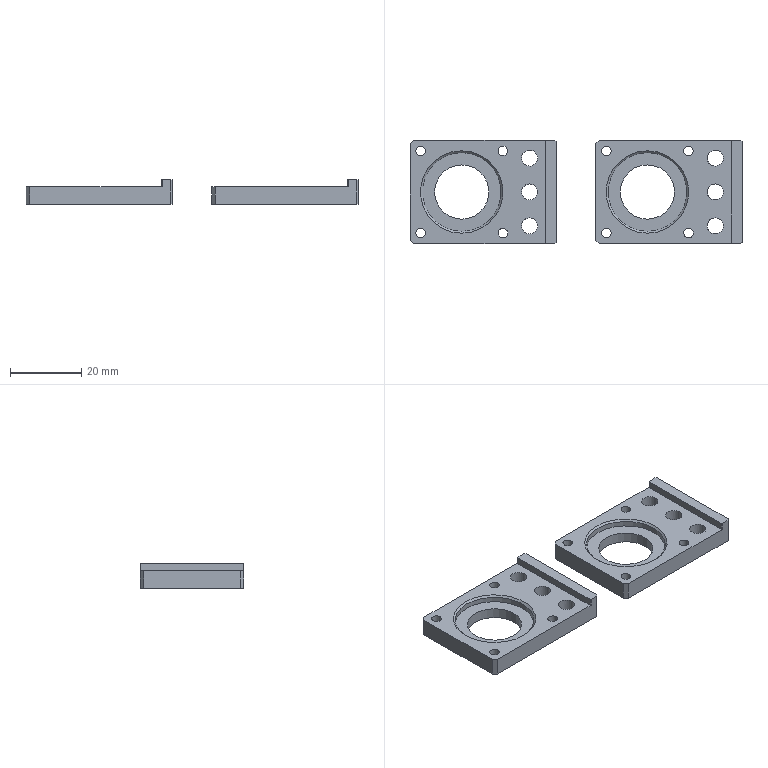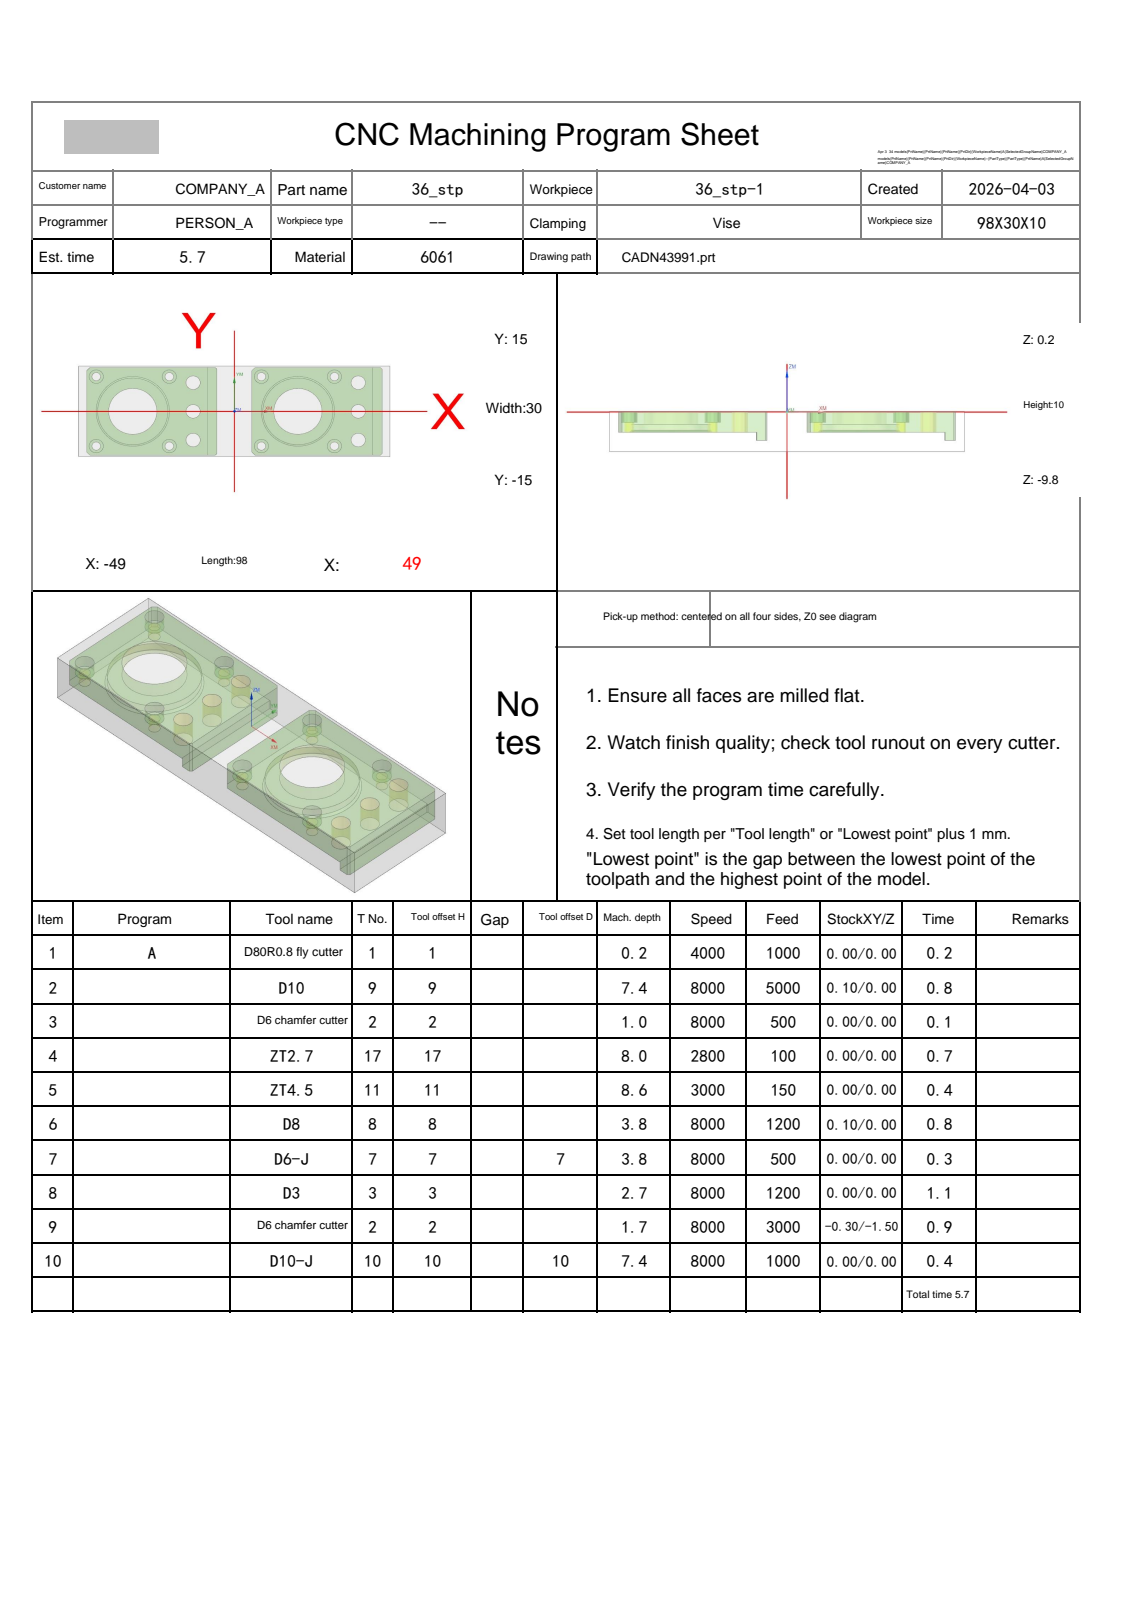NC program | NX | posted by the shop | part box 93 x 29 x 7 mm
Whole program, first 1395 of 1759 lines:
%
O0001
(Machine time: 7.58 MIN)
(===Total Tool:9===)
(T1=D80R0.8 fly cutter D=80.  R=0.8  D-  H01 Z=0.    )
(T9=D10     D=10.  R=0.   D-  H09 Z=-7.2  )
(T2=D6 chamfer cutter   D=6.   R=0.   D-  H02 Z=-1.5  )
(T17=ZT2.7  D=2.7  DR_a=120 D-  H17 Z=-7.78 )
(T11=ZT4.5  D=4.5  DR_a=118 D-  H11 Z=-8.35 )
(T8=D8      D=8.   R=0.   D-  H08 Z=-3.58 )
(T7=D6-J    D=6.   R=0.   D7  H07 Z=-3.58 )
(T3=D3      D=3.   R=0.   D3  H03 Z=-2.5  )
(T10=D10-J  D=10.  R=0.   D10 H10 Z=-7.2  )
G80 G90 G17 G49 G40
G91 G28 Z0
M01
N1 T01 M06
(D80R0.8 fly cutter  D=80. R=0.8 H=01 ce=0.00 di=0.00)
G00 G90 G54 X91.5 Y0.0 M03 S4000
G43 H01 Z20.
M08
Z2.
G01 Z0.0 F1000.
X86.5
X-86.5
X-91.5
Z2.
G00 Z20.
G91 G28 Z0.0
M05
M09
G91 G28 Z0.0
M01
N2 T09 M06
(D10  D=10. R=0. H=09 ce=0.10 di=0.00)
G00 G90 G54 X-25.75 Y-19.6 M03 S8000
G43 H09 Z20.
M08
Z.5
G01 X-45.5 Z.411 F5000.
G02 X-49.106 Y-18.106 Z.393 I0.0 J5.1
G01 X-50.106 Y-17.106 Z.386
G02 X-51.6 Y-13.5 Z.368 I3.606 J3.606
G01 Y13.5 Z.246
G02 X-50.106 Y17.106 Z.228 I5.1 J0.0
G01 X-49.106 Y18.106 Z.221
G02 X-45.5 Y19.6 Z.203 I3.606 J-3.606
G01 X-6. Z.025
G02 X-2.394 Y18.106 Z.007 I0.0 J-5.1
G01 X-1.894 Y17.606 Z.003
G02 X-.4 Y14. Z-.015 I-3.606 J-3.606
G01 Y-14. Z-.141
G02 X-1.894 Y-17.606 Z-.159 I-5.1 J0.0
G01 X-2.394 Y-18.106 Z-.163
G02 X-6. Y-19.6 Z-.181 I-3.606 J3.606
G01 X-45.5 Z-.359
G02 X-49.106 Y-18.106 Z-.377 I0.0 J5.1
G01 X-50.106 Y-17.106 Z-.384
G02 X-51.6 Y-13.5 Z-.402 I3.606 J3.606
G01 Y13.5 Z-.524
G02 X-50.106 Y17.106 Z-.542 I5.1 J0.0
G01 X-49.106 Y18.106 Z-.549
G02 X-45.5 Y19.6 Z-.567 I3.606 J-3.606
G01 X-6. Z-.745
G02 X-2.394 Y18.106 Z-.763 I0.0 J-5.1
G01 X-1.894 Y17.606 Z-.767
G02 X-.4 Y14. Z-.785 I-3.606 J-3.606
G01 Y-14. Z-.911
G02 X-1.894 Y-17.606 Z-.929 I-5.1 J0.0
G01 X-2.394 Y-18.106 Z-.933
G02 X-6. Y-19.6 Z-.951 I-3.606 J3.606
G01 X-45.5 Z-1.129
G02 X-49.106 Y-18.106 Z-1.147 I0.0 J5.1
G01 X-50.106 Y-17.106 Z-1.154
G02 X-51.6 Y-13.5 Z-1.172 I3.606 J3.606
G01 Y13.5 Z-1.294
G02 X-50.106 Y17.106 Z-1.312 I5.1 J0.0
G01 X-49.106 Y18.106 Z-1.319
G02 X-45.5 Y19.6 Z-1.337 I3.606 J-3.606
G01 X-6. Z-1.515
G02 X-2.394 Y18.106 Z-1.533 I0.0 J-5.1
G01 X-1.894 Y17.606 Z-1.537
G02 X-.4 Y14. Z-1.555 I-3.606 J-3.606
G01 Y-14. Z-1.681
G02 X-1.894 Y-17.606 Z-1.699 I-5.1 J0.0
G01 X-2.394 Y-18.106 Z-1.703
G02 X-6. Y-19.6 Z-1.721 I-3.606 J3.606
G01 X-45.5 Z-1.899
G02 X-49.106 Y-18.106 Z-1.917 I0.0 J5.1
G01 X-50.106 Y-17.106 Z-1.924
G02 X-51.6 Y-13.5 Z-1.942 I3.606 J3.606
G01 Y13.5 Z-2.064
G02 X-50.106 Y17.106 Z-2.082 I5.1 J0.0
G01 X-49.106 Y18.106 Z-2.089
G02 X-45.5 Y19.6 Z-2.107 I3.606 J-3.606
G01 X-6. Z-2.285
G02 X-2.394 Y18.106 Z-2.303 I0.0 J-5.1
G01 X-1.894 Y17.606 Z-2.307
G02 X-.4 Y14. Z-2.325 I-3.606 J-3.606
G01 Y-14. Z-2.451
G02 X-1.894 Y-17.606 Z-2.469 I-5.1 J0.0
G01 X-2.394 Y-18.106 Z-2.473
G02 X-6. Y-19.6 Z-2.491 I-3.606 J3.606
G01 X-45.5 Z-2.669
G02 X-49.106 Y-18.106 Z-2.687 I0.0 J5.1
G01 X-50.106 Y-17.106 Z-2.694
G02 X-51.6 Y-13.5 Z-2.712 I3.606 J3.606
G01 Y13.5 Z-2.834
G02 X-50.106 Y17.106 Z-2.852 I5.1 J0.0
G01 X-49.106 Y18.106 Z-2.859
G02 X-45.5 Y19.6 Z-2.877 I3.606 J-3.606
G01 X-6. Z-3.055
G02 X-2.394 Y18.106 Z-3.073 I0.0 J-5.1
G01 X-1.894 Y17.606 Z-3.077
G02 X-.4 Y14. Z-3.095 I-3.606 J-3.606
G01 Y-14. Z-3.221
G02 X-1.894 Y-17.606 Z-3.239 I-5.1 J0.0
G01 X-2.394 Y-18.106 Z-3.243
G02 X-6. Y-19.6 Z-3.261 I-3.606 J3.606
G01 X-45.5 Z-3.439
G02 X-49.106 Y-18.106 Z-3.457 I0.0 J5.1
G01 X-50.106 Y-17.106 Z-3.464
G02 X-51.6 Y-13.5 Z-3.482 I3.606 J3.606
G01 Y13.5 Z-3.604
G02 X-50.106 Y17.106 Z-3.622 I5.1 J0.0
G01 X-49.106 Y18.106 Z-3.629
G02 X-45.5 Y19.6 Z-3.647 I3.606 J-3.606
G01 X-6. Z-3.825
G02 X-2.394 Y18.106 Z-3.843 I0.0 J-5.1
G01 X-1.894 Y17.606 Z-3.847
G02 X-.4 Y14. Z-3.865 I-3.606 J-3.606
G01 Y-14. Z-3.991
G02 X-1.894 Y-17.606 Z-4.009 I-5.1 J0.0
G01 X-2.394 Y-18.106 Z-4.013
G02 X-6. Y-19.6 Z-4.031 I-3.606 J3.606
G01 X-45.5 Z-4.209
G02 X-49.106 Y-18.106 Z-4.227 I0.0 J5.1
G01 X-50.106 Y-17.106 Z-4.234
G02 X-51.6 Y-13.5 Z-4.252 I3.606 J3.606
G01 Y13.5 Z-4.374
G02 X-50.106 Y17.106 Z-4.392 I5.1 J0.0
G01 X-49.106 Y18.106 Z-4.399
G02 X-45.5 Y19.6 Z-4.417 I3.606 J-3.606
G01 X-6. Z-4.595
G02 X-2.394 Y18.106 Z-4.613 I0.0 J-5.1
G01 X-1.894 Y17.606 Z-4.617
G02 X-.4 Y14. Z-4.635 I-3.606 J-3.606
G01 Y-14. Z-4.761
G02 X-1.894 Y-17.606 Z-4.779 I-5.1 J0.0
G01 X-2.394 Y-18.106 Z-4.783
G02 X-6. Y-19.6 Z-4.801 I-3.606 J3.606
G01 X-45.5 Z-4.979
G02 X-49.106 Y-18.106 Z-4.997 I0.0 J5.1
G01 X-50.106 Y-17.106 Z-5.004
G02 X-51.6 Y-13.5 Z-5.022 I3.606 J3.606
G01 Y13.5 Z-5.144
G02 X-50.106 Y17.106 Z-5.162 I5.1 J0.0
G01 X-49.106 Y18.106 Z-5.169
G02 X-45.5 Y19.6 Z-5.187 I3.606 J-3.606
G01 X-6. Z-5.365
G02 X-2.394 Y18.106 Z-5.383 I0.0 J-5.1
G01 X-1.894 Y17.606 Z-5.387
G02 X-.4 Y14. Z-5.405 I-3.606 J-3.606
G01 Y-14. Z-5.531
G02 X-1.894 Y-17.606 Z-5.549 I-5.1 J0.0
G01 X-2.394 Y-18.106 Z-5.553
G02 X-6. Y-19.6 Z-5.571 I-3.606 J3.606
G01 X-45.5 Z-5.749
G02 X-49.106 Y-18.106 Z-5.767 I0.0 J5.1
G01 X-50.106 Y-17.106 Z-5.774
G02 X-51.6 Y-13.5 Z-5.792 I3.606 J3.606
G01 Y13.5 Z-5.914
G02 X-50.106 Y17.106 Z-5.932 I5.1 J0.0
G01 X-49.106 Y18.106 Z-5.939
G02 X-45.5 Y19.6 Z-5.957 I3.606 J-3.606
G01 X-6. Z-6.135
G02 X-2.394 Y18.106 Z-6.153 I0.0 J-5.1
G01 X-1.894 Y17.606 Z-6.157
G02 X-.4 Y14. Z-6.175 I-3.606 J-3.606
G01 Y-14. Z-6.301
G02 X-1.894 Y-17.606 Z-6.319 I-5.1 J0.0
G01 X-2.394 Y-18.106 Z-6.323
G02 X-6. Y-19.6 Z-6.341 I-3.606 J3.606
G01 X-45.5 Z-6.519
G02 X-49.106 Y-18.106 Z-6.537 I0.0 J5.1
G01 X-50.106 Y-17.106 Z-6.544
G02 X-51.6 Y-13.5 Z-6.562 I3.606 J3.606
G01 Y13.5 Z-6.684
G02 X-50.106 Y17.106 Z-6.702 I5.1 J0.0
G01 X-49.106 Y18.106 Z-6.709
G02 X-45.5 Y19.6 Z-6.727 I3.606 J-3.606
G01 X-6. Z-6.905
G02 X-2.394 Y18.106 Z-6.923 I0.0 J-5.1
G01 X-1.894 Y17.606 Z-6.927
G02 X-.4 Y14. Z-6.945 I-3.606 J-3.606
G01 Y-14. Z-7.071
G02 X-1.894 Y-17.606 Z-7.089 I-5.1 J0.0
G01 X-2.394 Y-18.106 Z-7.093
G02 X-6. Y-19.6 Z-7.111 I-3.606 J3.606
G01 X-25.75 Z-7.2
X-45.5
G02 X-49.106 Y-18.106 I0.0 J5.1
G01 X-50.106 Y-17.106
G02 X-51.6 Y-13.5 I3.606 J3.606
G01 Y13.5
G02 X-50.106 Y17.106 I5.1 J0.0
G01 X-49.106 Y18.106
G02 X-45.5 Y19.6 I3.606 J-3.606
G01 X-6.
G02 X-2.394 Y18.106 I0.0 J-5.1
G01 X-1.894 Y17.606
G02 X-.4 Y14. I-3.606 J-3.606
G01 Y-14.
G02 X-1.894 Y-17.606 I-5.1 J0.0
G01 X-2.394 Y-18.106
G02 X-6. Y-19.6 I-3.606 J3.606
G01 X-25.75
X-26.25
Z-6.2
G00 Z20.
X26.25
Z.5
G01 X6.5 Z.411
G02 X2.894 Y-18.106 Z.393 I0.0 J5.1
G01 X1.894 Y-17.106 Z.386
G02 X.4 Y-13.5 Z.368 I3.606 J3.606
G01 Y13.5 Z.246
G02 X1.894 Y17.106 Z.228 I5.1 J0.0
G01 X2.894 Y18.106 Z.221
G02 X6.5 Y19.6 Z.203 I3.606 J-3.606
G01 X46. Z.025
G02 X49.606 Y18.106 Z.007 I0.0 J-5.1
G01 X50.106 Y17.606 Z.003
G02 X51.6 Y14. Z-.015 I-3.606 J-3.606
G01 Y-14. Z-.141
G02 X50.106 Y-17.606 Z-.159 I-5.1 J0.0
G01 X49.606 Y-18.106 Z-.163
G02 X46. Y-19.6 Z-.181 I-3.606 J3.606
G01 X6.5 Z-.359
G02 X2.894 Y-18.106 Z-.377 I0.0 J5.1
G01 X1.894 Y-17.106 Z-.384
G02 X.4 Y-13.5 Z-.402 I3.606 J3.606
G01 Y13.5 Z-.524
G02 X1.894 Y17.106 Z-.542 I5.1 J0.0
G01 X2.894 Y18.106 Z-.549
G02 X6.5 Y19.6 Z-.567 I3.606 J-3.606
G01 X46. Z-.745
G02 X49.606 Y18.106 Z-.763 I0.0 J-5.1
G01 X50.106 Y17.606 Z-.767
G02 X51.6 Y14. Z-.785 I-3.606 J-3.606
G01 Y-14. Z-.911
G02 X50.106 Y-17.606 Z-.929 I-5.1 J0.0
G01 X49.606 Y-18.106 Z-.933
G02 X46. Y-19.6 Z-.951 I-3.606 J3.606
G01 X6.5 Z-1.129
G02 X2.894 Y-18.106 Z-1.147 I0.0 J5.1
G01 X1.894 Y-17.106 Z-1.154
G02 X.4 Y-13.5 Z-1.172 I3.606 J3.606
G01 Y13.5 Z-1.294
G02 X1.894 Y17.106 Z-1.312 I5.1 J0.0
G01 X2.894 Y18.106 Z-1.319
G02 X6.5 Y19.6 Z-1.337 I3.606 J-3.606
G01 X46. Z-1.515
G02 X49.606 Y18.106 Z-1.533 I0.0 J-5.1
G01 X50.106 Y17.606 Z-1.537
G02 X51.6 Y14. Z-1.555 I-3.606 J-3.606
G01 Y-14. Z-1.681
G02 X50.106 Y-17.606 Z-1.699 I-5.1 J0.0
G01 X49.606 Y-18.106 Z-1.703
G02 X46. Y-19.6 Z-1.721 I-3.606 J3.606
G01 X6.5 Z-1.899
G02 X2.894 Y-18.106 Z-1.917 I0.0 J5.1
G01 X1.894 Y-17.106 Z-1.924
G02 X.4 Y-13.5 Z-1.942 I3.606 J3.606
G01 Y13.5 Z-2.064
G02 X1.894 Y17.106 Z-2.082 I5.1 J0.0
G01 X2.894 Y18.106 Z-2.089
G02 X6.5 Y19.6 Z-2.107 I3.606 J-3.606
G01 X46. Z-2.285
G02 X49.606 Y18.106 Z-2.303 I0.0 J-5.1
G01 X50.106 Y17.606 Z-2.307
G02 X51.6 Y14. Z-2.325 I-3.606 J-3.606
G01 Y-14. Z-2.451
G02 X50.106 Y-17.606 Z-2.469 I-5.1 J0.0
G01 X49.606 Y-18.106 Z-2.473
G02 X46. Y-19.6 Z-2.491 I-3.606 J3.606
G01 X6.5 Z-2.669
G02 X2.894 Y-18.106 Z-2.687 I0.0 J5.1
G01 X1.894 Y-17.106 Z-2.694
G02 X.4 Y-13.5 Z-2.712 I3.606 J3.606
G01 Y13.5 Z-2.834
G02 X1.894 Y17.106 Z-2.852 I5.1 J0.0
G01 X2.894 Y18.106 Z-2.859
G02 X6.5 Y19.6 Z-2.877 I3.606 J-3.606
G01 X46. Z-3.055
G02 X49.606 Y18.106 Z-3.073 I0.0 J-5.1
G01 X50.106 Y17.606 Z-3.077
G02 X51.6 Y14. Z-3.095 I-3.606 J-3.606
G01 Y-14. Z-3.221
G02 X50.106 Y-17.606 Z-3.239 I-5.1 J0.0
G01 X49.606 Y-18.106 Z-3.243
G02 X46. Y-19.6 Z-3.261 I-3.606 J3.606
G01 X6.5 Z-3.439
G02 X2.894 Y-18.106 Z-3.457 I0.0 J5.1
G01 X1.894 Y-17.106 Z-3.464
G02 X.4 Y-13.5 Z-3.482 I3.606 J3.606
G01 Y13.5 Z-3.604
G02 X1.894 Y17.106 Z-3.622 I5.1 J0.0
G01 X2.894 Y18.106 Z-3.629
G02 X6.5 Y19.6 Z-3.647 I3.606 J-3.606
G01 X46. Z-3.825
G02 X49.606 Y18.106 Z-3.843 I0.0 J-5.1
G01 X50.106 Y17.606 Z-3.847
G02 X51.6 Y14. Z-3.865 I-3.606 J-3.606
G01 Y-14. Z-3.991
G02 X50.106 Y-17.606 Z-4.009 I-5.1 J0.0
G01 X49.606 Y-18.106 Z-4.013
G02 X46. Y-19.6 Z-4.031 I-3.606 J3.606
G01 X6.5 Z-4.209
G02 X2.894 Y-18.106 Z-4.227 I0.0 J5.1
G01 X1.894 Y-17.106 Z-4.234
G02 X.4 Y-13.5 Z-4.252 I3.606 J3.606
G01 Y13.5 Z-4.374
G02 X1.894 Y17.106 Z-4.392 I5.1 J0.0
G01 X2.894 Y18.106 Z-4.399
G02 X6.5 Y19.6 Z-4.417 I3.606 J-3.606
G01 X46. Z-4.595
G02 X49.606 Y18.106 Z-4.613 I0.0 J-5.1
G01 X50.106 Y17.606 Z-4.617
G02 X51.6 Y14. Z-4.635 I-3.606 J-3.606
G01 Y-14. Z-4.761
G02 X50.106 Y-17.606 Z-4.779 I-5.1 J0.0
G01 X49.606 Y-18.106 Z-4.783
G02 X46. Y-19.6 Z-4.801 I-3.606 J3.606
G01 X6.5 Z-4.979
G02 X2.894 Y-18.106 Z-4.997 I0.0 J5.1
G01 X1.894 Y-17.106 Z-5.004
G02 X.4 Y-13.5 Z-5.022 I3.606 J3.606
G01 Y13.5 Z-5.144
G02 X1.894 Y17.106 Z-5.162 I5.1 J0.0
G01 X2.894 Y18.106 Z-5.169
G02 X6.5 Y19.6 Z-5.187 I3.606 J-3.606
G01 X46. Z-5.365
G02 X49.606 Y18.106 Z-5.383 I0.0 J-5.1
G01 X50.106 Y17.606 Z-5.387
G02 X51.6 Y14. Z-5.405 I-3.606 J-3.606
G01 Y-14. Z-5.531
G02 X50.106 Y-17.606 Z-5.549 I-5.1 J0.0
G01 X49.606 Y-18.106 Z-5.553
G02 X46. Y-19.6 Z-5.571 I-3.606 J3.606
G01 X6.5 Z-5.749
G02 X2.894 Y-18.106 Z-5.767 I0.0 J5.1
G01 X1.894 Y-17.106 Z-5.774
G02 X.4 Y-13.5 Z-5.792 I3.606 J3.606
G01 Y13.5 Z-5.914
G02 X1.894 Y17.106 Z-5.932 I5.1 J0.0
G01 X2.894 Y18.106 Z-5.939
G02 X6.5 Y19.6 Z-5.957 I3.606 J-3.606
G01 X46. Z-6.135
G02 X49.606 Y18.106 Z-6.153 I0.0 J-5.1
G01 X50.106 Y17.606 Z-6.157
G02 X51.6 Y14. Z-6.175 I-3.606 J-3.606
G01 Y-14. Z-6.301
G02 X50.106 Y-17.606 Z-6.319 I-5.1 J0.0
G01 X49.606 Y-18.106 Z-6.323
G02 X46. Y-19.6 Z-6.341 I-3.606 J3.606
G01 X6.5 Z-6.519
G02 X2.894 Y-18.106 Z-6.537 I0.0 J5.1
G01 X1.894 Y-17.106 Z-6.544
G02 X.4 Y-13.5 Z-6.562 I3.606 J3.606
G01 Y13.5 Z-6.684
G02 X1.894 Y17.106 Z-6.702 I5.1 J0.0
G01 X2.894 Y18.106 Z-6.709
G02 X6.5 Y19.6 Z-6.727 I3.606 J-3.606
G01 X46. Z-6.905
G02 X49.606 Y18.106 Z-6.923 I0.0 J-5.1
G01 X50.106 Y17.606 Z-6.927
G02 X51.6 Y14. Z-6.945 I-3.606 J-3.606
G01 Y-14. Z-7.071
G02 X50.106 Y-17.606 Z-7.089 I-5.1 J0.0
G01 X49.606 Y-18.106 Z-7.093
G02 X46. Y-19.6 Z-7.111 I-3.606 J3.606
G01 X26.25 Z-7.2
X6.5
G02 X2.894 Y-18.106 I0.0 J5.1
G01 X1.894 Y-17.106
G02 X.4 Y-13.5 I3.606 J3.606
G01 Y13.5
G02 X1.894 Y17.106 I5.1 J0.0
G01 X2.894 Y18.106
G02 X6.5 Y19.6 I3.606 J-3.606
G01 X46.
G02 X49.606 Y18.106 I0.0 J-5.1
G01 X50.106 Y17.606
G02 X51.6 Y14. I-3.606 J-3.606
G01 Y-14.
G02 X50.106 Y-17.606 I-5.1 J0.0
G01 X49.606 Y-18.106
G02 X46. Y-19.6 I-3.606 J3.606
G01 X26.25
X25.75
Z-6.2
G00 Z20.
G91 G28 Z0.0
M05
M09
G91 G28 Z0.0
M01
N3 T02 M06
(D6 chamfer cutter  D=6. R=0. H=02 ce=0.00 di=0.00)
G00 G90 G54 X-43.5 Y-11.5 M03 S8000
G43 H02 Z20.
M08
G98 G81 X-43.5 Y-11.5 Z-.8 R1. F500.
Y11.5
X-32. Y0.0
X-20.5 Y11.5
X-13. Y9.5
Y0.0
X-20.5 Y-11.5
X-13. Y-9.5
X8.5 Y-11.5
X20. Y0.0
X31.5 Y-11.5
X39. Y-9.5
Y0.0
Y9.5
X31.5 Y11.5
X8.5
G80
G00 Z20.
G91 G28 Z0.0
M05
M09
G91 G28 Z0.0
M01
N4 T17 M06
(ZT2.7 D=2.7 DR_a=120 H=17)
G00 G90 G54 X-20.5 Y-11.5 M03 S2800
G43 H17 Z20.
M08
G98 G83 X-20.5 Y-11.5 Z-7.779 R1. F100. Q2.
X-43.5
Y11.5
X-20.5
X8.5
Y-11.5
X31.5
Y11.5
G80
G00 Z20.
G91 G28 Z0.0
M05
M09
G91 G28 Z0.0
M01
N5 T11 M06
(ZT4.5 D=4.5 DR_a=118 H=11)
G00 G90 G54 X-13. Y9.5 M03 S3000
G43 H11 Z20.
M08
G98 G83 X-13. Y9.5 Z-8.352 R1. F150. Q3.
Y0.0
Y-9.5
X39.
Y0.0
Y9.5
G80
G00 Z20.
G91 G28 Z0.0
M05
M09
G91 G28 Z0.0
M01
N6 T08 M06
(D8  D=8. R=0. H=08 ce=0.10 di=0.00)
G00 G90 G54 X-32. Y0.0 M03 S8000
G43 H08 Z20.
M08
Z.5
G03 X-30.25 Y-1.75 I1.75 J0.0 F1200.
X-28.5 Y0.0 I0.0 J1.75
X-28.5 Y0.0 Z.3 I-3.5 J0.0
X-28.5 Y0.0 Z.1 I-3.5 J0.0
X-28.5 Y0.0 Z-.1 I-3.5 J0.0
X-28.5 Y0.0 Z-.3 I-3.5 J0.0
X-28.5 Y0.0 Z-.5 I-3.5 J0.0
X-28.5 Y0.0 Z-.7 I-3.5 J0.0
X-28.5 Y0.0 Z-.9 I-3.5 J0.0
X-28.5 Y0.0 Z-1.1 I-3.5 J0.0
X-28.5 Y0.0 Z-1.3 I-3.5 J0.0
X-28.5 Y0.0 Z-1.5 I-3.5 J0.0
X-28.5 Y0.0 Z-1.7 I-3.5 J0.0
X-28.5 Y0.0 Z-1.9 I-3.5 J0.0
X-28.5 Y0.0 Z-2.1 I-3.5 J0.0
X-28.5 Y0.0 Z-2.3 I-3.5 J0.0
X-28.5 Y0.0 Z-2.5 I-3.5 J0.0
X-28.5 Y0.0 Z-2.7 I-3.5 J0.0
X-28.5 Y0.0 Z-2.9 I-3.5 J0.0
X-28.5 Y0.0 Z-3.1 I-3.5 J0.0
X-28.5 Y0.0 Z-3.3 I-3.5 J0.0
X-28.5 Y0.0 Z-3.5 I-3.5 J0.0
X-34.832 Y2.057 Z-3.58 I-3.5 J0.0
X-35.5 Y0.0 I2.832 J-2.057
X-32. Y-3.5 I3.5 J0.0
X-28.5 Y0.0 I0.0 J3.5
X-32. Y3.5 I-3.5 J0.0
X-34.832 Y2.057 I0.0 J-3.5
X-35.166 Y1.029 I1.416 J-1.029
X-33.416 Y-.721 I1.75 J0.0
X-32. Y0.0 I0.0 J1.75
G00 Z20.
X20.
Z.5
G03 X21.75 Y-1.75 I1.75 J0.0
X23.5 Y0.0 I0.0 J1.75
X23.5 Y0.0 Z.3 I-3.5 J0.0
X23.5 Y0.0 Z.1 I-3.5 J0.0
X23.5 Y0.0 Z-.1 I-3.5 J0.0
X23.5 Y0.0 Z-.3 I-3.5 J0.0
X23.5 Y0.0 Z-.5 I-3.5 J0.0
X23.5 Y0.0 Z-.7 I-3.5 J0.0
X23.5 Y0.0 Z-.9 I-3.5 J0.0
X23.5 Y0.0 Z-1.1 I-3.5 J0.0
X23.5 Y0.0 Z-1.3 I-3.5 J0.0
X23.5 Y0.0 Z-1.5 I-3.5 J0.0
X23.5 Y0.0 Z-1.7 I-3.5 J0.0
X23.5 Y0.0 Z-1.9 I-3.5 J0.0
X23.5 Y0.0 Z-2.1 I-3.5 J0.0
X23.5 Y0.0 Z-2.3 I-3.5 J0.0
X23.5 Y0.0 Z-2.5 I-3.5 J0.0
X23.5 Y0.0 Z-2.7 I-3.5 J0.0
X23.5 Y0.0 Z-2.9 I-3.5 J0.0
X23.5 Y0.0 Z-3.1 I-3.5 J0.0
X23.5 Y0.0 Z-3.3 I-3.5 J0.0
X23.5 Y0.0 Z-3.5 I-3.5 J0.0
X17.168 Y2.057 Z-3.58 I-3.5 J0.0
X16.5 Y0.0 I2.832 J-2.057
X20. Y-3.5 I3.5 J0.0
X23.5 Y0.0 I0.0 J3.5
X20. Y3.5 I-3.5 J0.0
X17.168 Y2.057 I0.0 J-3.5
X16.834 Y1.029 I1.416 J-1.029
X18.584 Y-.721 I1.75 J0.0
X20. Y0.0 I0.0 J1.75
G00 Z20.
G91 G28 Z0.0
M05
M09
G91 G28 Z0.0
M01
N7 T07 M06
(D6-J  D=6. R=0. H=07 ce=0.00 di=0.00)
G00 G90 G54 X-32. Y0.0 M03 S8000
G43 H07 Z20.
M08
Z.5
G41 D07
G01 X-31.116 Y-1.212 F500.
G03 X-29.455 Y-2.055 I1.66 J1.212
X-27.4 Y0.0 I0.0 J2.055
X-30.147 Y-4.21 Z-3.58 I-4.6 J0.0
X-27.4 Y0.0 I-1.853 J4.21
X-32. Y4.6 I-4.6 J0.0
X-36.6 Y0.0 I0.0 J-4.6
X-32. Y-4.6 I4.6 J0.0
X-30.147 Y-4.21 I0.0 J4.6
X-28.919 Y-2.329 I-.828 J1.881
X-30.535 Y-.321 I-2.055 J0.0
G01 G40 X-32. Y0.0
G00 Z20.
X20.
Z.5
G41 D07
G01 X20.884 Y-1.212
G03 X22.545 Y-2.055 I1.66 J1.212
X24.6 Y0.0 I0.0 J2.055
X21.853 Y-4.21 Z-3.58 I-4.6 J0.0
X24.6 Y0.0 I-1.853 J4.21
X20. Y4.6 I-4.6 J0.0
X15.4 Y0.0 I0.0 J-4.6
X20. Y-4.6 I4.6 J0.0
X21.853 Y-4.21 I0.0 J4.6
X23.081 Y-2.329 I-.828 J1.881
X21.465 Y-.321 I-2.055 J0.0
G01 G40 X20. Y0.0
G00 Z20.
G91 G28 Z0.0
M05
M09
G91 G28 Z0.0
M01
N8 T03 M06
(D3  D=3. R=0. H=03 ce=0.10 di=0.00)
G00 G90 G54 X-20.5 Y11.5 M03 S8000
G43 H03 Z20.
M08
Z.5
G03 X-20.175 Y11.175 I.325 J0.0 F1200.
X-19.85 Y11.5 I0.0 J.325
X-19.85 Y11.5 Z.4 I-.65 J0.0
X-19.85 Y11.5 Z.3 I-.65 J0.0
X-19.85 Y11.5 Z.2 I-.65 J0.0
X-19.85 Y11.5 Z.1 I-.65 J0.0
X-19.85 Y11.5 Z0.0 I-.65 J0.0
X-19.85 Y11.5 Z-.1 I-.65 J0.0
X-19.85 Y11.5 Z-.2 I-.65 J0.0
X-19.85 Y11.5 Z-.3 I-.65 J0.0
X-19.85 Y11.5 Z-.4 I-.65 J0.0
X-19.85 Y11.5 Z-.5 I-.65 J0.0
X-19.85 Y11.5 Z-.6 I-.65 J0.0
X-19.85 Y11.5 Z-.7 I-.65 J0.0
X-19.85 Y11.5 Z-.8 I-.65 J0.0
X-19.85 Y11.5 Z-.9 I-.65 J0.0
X-19.85 Y11.5 Z-1. I-.65 J0.0
X-19.85 Y11.5 Z-1.1 I-.65 J0.0
X-19.85 Y11.5 Z-1.2 I-.65 J0.0
X-19.85 Y11.5 Z-1.3 I-.65 J0.0
X-19.85 Y11.5 Z-1.4 I-.65 J0.0
X-19.85 Y11.5 Z-1.5 I-.65 J0.0
X-19.85 Y11.5 Z-1.6 I-.65 J0.0
X-19.85 Y11.5 Z-1.7 I-.65 J0.0
X-19.85 Y11.5 Z-1.8 I-.65 J0.0
X-19.85 Y11.5 Z-1.9 I-.65 J0.0
X-19.85 Y11.5 Z-2. I-.65 J0.0
X-19.85 Y11.5 Z-2.1 I-.65 J0.0
X-19.85 Y11.5 Z-2.2 I-.65 J0.0
X-19.85 Y11.5 Z-2.3 I-.65 J0.0
X-19.85 Y11.5 Z-2.4 I-.65 J0.0
X-19.85 Y11.5 Z-2.5 I-.65 J0.0
X-20.5 Y12.15 I-.65 J0.0
X-21.15 Y11.5 I0.0 J-.65
X-20.5 Y10.85 I.65 J0.0
X-19.85 Y11.5 I0.0 J.65
X-20.175 Y11.825 I-.325 J0.0
X-20.5 Y11.5 I0.0 J-.325
G00 Z20.
X-43.5
Z.5
G03 X-43.175 Y11.175 I.325 J0.0
X-42.85 Y11.5 I0.0 J.325
X-42.85 Y11.5 Z.4 I-.65 J0.0
X-42.85 Y11.5 Z.3 I-.65 J0.0
X-42.85 Y11.5 Z.2 I-.65 J0.0
X-42.85 Y11.5 Z.1 I-.65 J0.0
X-42.85 Y11.5 Z0.0 I-.65 J0.0
X-42.85 Y11.5 Z-.1 I-.65 J0.0
X-42.85 Y11.5 Z-.2 I-.65 J0.0
X-42.85 Y11.5 Z-.3 I-.65 J0.0
X-42.85 Y11.5 Z-.4 I-.65 J0.0
X-42.85 Y11.5 Z-.5 I-.65 J0.0
X-42.85 Y11.5 Z-.6 I-.65 J0.0
X-42.85 Y11.5 Z-.7 I-.65 J0.0
X-42.85 Y11.5 Z-.8 I-.65 J0.0
X-42.85 Y11.5 Z-.9 I-.65 J0.0
X-42.85 Y11.5 Z-1. I-.65 J0.0
X-42.85 Y11.5 Z-1.1 I-.65 J0.0
X-42.85 Y11.5 Z-1.2 I-.65 J0.0
X-42.85 Y11.5 Z-1.3 I-.65 J0.0
X-42.85 Y11.5 Z-1.4 I-.65 J0.0
X-42.85 Y11.5 Z-1.5 I-.65 J0.0
X-42.85 Y11.5 Z-1.6 I-.65 J0.0
X-42.85 Y11.5 Z-1.7 I-.65 J0.0
X-42.85 Y11.5 Z-1.8 I-.65 J0.0
X-42.85 Y11.5 Z-1.9 I-.65 J0.0
X-42.85 Y11.5 Z-2. I-.65 J0.0
X-42.85 Y11.5 Z-2.1 I-.65 J0.0
X-42.85 Y11.5 Z-2.2 I-.65 J0.0
X-42.85 Y11.5 Z-2.3 I-.65 J0.0
X-42.85 Y11.5 Z-2.4 I-.65 J0.0
X-42.85 Y11.5 Z-2.5 I-.65 J0.0
X-43.5 Y12.15 I-.65 J0.0
X-44.15 Y11.5 I0.0 J-.65
X-43.5 Y10.85 I.65 J0.0
X-42.85 Y11.5 I0.0 J.65
X-43.175 Y11.825 I-.325 J0.0
X-43.5 Y11.5 I0.0 J-.325
G00 Z20.
Y-11.5
Z.5
G03 X-43.175 Y-11.825 I.325 J0.0
X-42.85 Y-11.5 I0.0 J.325
X-42.85 Y-11.5 Z.4 I-.65 J0.0
X-42.85 Y-11.5 Z.3 I-.65 J0.0
X-42.85 Y-11.5 Z.2 I-.65 J0.0
X-42.85 Y-11.5 Z.1 I-.65 J0.0
X-42.85 Y-11.5 Z0.0 I-.65 J0.0
X-42.85 Y-11.5 Z-.1 I-.65 J0.0
X-42.85 Y-11.5 Z-.2 I-.65 J0.0
X-42.85 Y-11.5 Z-.3 I-.65 J0.0
X-42.85 Y-11.5 Z-.4 I-.65 J0.0
X-42.85 Y-11.5 Z-.5 I-.65 J0.0
X-42.85 Y-11.5 Z-.6 I-.65 J0.0
X-42.85 Y-11.5 Z-.7 I-.65 J0.0
X-42.85 Y-11.5 Z-.8 I-.65 J0.0
X-42.85 Y-11.5 Z-.9 I-.65 J0.0
X-42.85 Y-11.5 Z-1. I-.65 J0.0
X-42.85 Y-11.5 Z-1.1 I-.65 J0.0
X-42.85 Y-11.5 Z-1.2 I-.65 J0.0
X-42.85 Y-11.5 Z-1.3 I-.65 J0.0
X-42.85 Y-11.5 Z-1.4 I-.65 J0.0
X-42.85 Y-11.5 Z-1.5 I-.65 J0.0
X-42.85 Y-11.5 Z-1.6 I-.65 J0.0
X-42.85 Y-11.5 Z-1.7 I-.65 J0.0
X-42.85 Y-11.5 Z-1.8 I-.65 J0.0
X-42.85 Y-11.5 Z-1.9 I-.65 J0.0
X-42.85 Y-11.5 Z-2. I-.65 J0.0
X-42.85 Y-11.5 Z-2.1 I-.65 J0.0
X-42.85 Y-11.5 Z-2.2 I-.65 J0.0
X-42.85 Y-11.5 Z-2.3 I-.65 J0.0
X-42.85 Y-11.5 Z-2.4 I-.65 J0.0
X-42.85 Y-11.5 Z-2.5 I-.65 J0.0
X-43.5 Y-10.85 I-.65 J0.0
X-44.15 Y-11.5 I0.0 J-.65
X-43.5 Y-12.15 I.65 J0.0
X-42.85 Y-11.5 I0.0 J.65
X-43.175 Y-11.175 I-.325 J0.0
X-43.5 Y-11.5 I0.0 J-.325
G00 Z20.
X-20.5
Z.5
G03 X-20.175 Y-11.825 I.325 J0.0
X-19.85 Y-11.5 I0.0 J.325
X-19.85 Y-11.5 Z.4 I-.65 J0.0
X-19.85 Y-11.5 Z.3 I-.65 J0.0
X-19.85 Y-11.5 Z.2 I-.65 J0.0
X-19.85 Y-11.5 Z.1 I-.65 J0.0
X-19.85 Y-11.5 Z0.0 I-.65 J0.0
X-19.85 Y-11.5 Z-.1 I-.65 J0.0
X-19.85 Y-11.5 Z-.2 I-.65 J0.0
X-19.85 Y-11.5 Z-.3 I-.65 J0.0
X-19.85 Y-11.5 Z-.4 I-.65 J0.0
X-19.85 Y-11.5 Z-.5 I-.65 J0.0
X-19.85 Y-11.5 Z-.6 I-.65 J0.0
X-19.85 Y-11.5 Z-.7 I-.65 J0.0
X-19.85 Y-11.5 Z-.8 I-.65 J0.0
X-19.85 Y-11.5 Z-.9 I-.65 J0.0
X-19.85 Y-11.5 Z-1. I-.65 J0.0
X-19.85 Y-11.5 Z-1.1 I-.65 J0.0
X-19.85 Y-11.5 Z-1.2 I-.65 J0.0
X-19.85 Y-11.5 Z-1.3 I-.65 J0.0
X-19.85 Y-11.5 Z-1.4 I-.65 J0.0
X-19.85 Y-11.5 Z-1.5 I-.65 J0.0
X-19.85 Y-11.5 Z-1.6 I-.65 J0.0
X-19.85 Y-11.5 Z-1.7 I-.65 J0.0
X-19.85 Y-11.5 Z-1.8 I-.65 J0.0
X-19.85 Y-11.5 Z-1.9 I-.65 J0.0
X-19.85 Y-11.5 Z-2. I-.65 J0.0
X-19.85 Y-11.5 Z-2.1 I-.65 J0.0
X-19.85 Y-11.5 Z-2.2 I-.65 J0.0
X-19.85 Y-11.5 Z-2.3 I-.65 J0.0
X-19.85 Y-11.5 Z-2.4 I-.65 J0.0
X-19.85 Y-11.5 Z-2.5 I-.65 J0.0
X-20.5 Y-10.85 I-.65 J0.0
X-21.15 Y-11.5 I0.0 J-.65
X-20.5 Y-12.15 I.65 J0.0
X-19.85 Y-11.5 I0.0 J.65
X-20.175 Y-11.175 I-.325 J0.0
X-20.5 Y-11.5 I0.0 J-.325
G00 Z20.
X8.5
Z.5
G03 X8.825 Y-11.825 I.325 J0.0
X9.15 Y-11.5 I0.0 J.325
X9.15 Y-11.5 Z.4 I-.65 J0.0
X9.15 Y-11.5 Z.3 I-.65 J0.0
X9.15 Y-11.5 Z.2 I-.65 J0.0
X9.15 Y-11.5 Z.1 I-.65 J0.0
X9.15 Y-11.5 Z0.0 I-.65 J0.0
X9.15 Y-11.5 Z-.1 I-.65 J0.0
X9.15 Y-11.5 Z-.2 I-.65 J0.0
X9.15 Y-11.5 Z-.3 I-.65 J0.0
X9.15 Y-11.5 Z-.4 I-.65 J0.0
X9.15 Y-11.5 Z-.5 I-.65 J0.0
X9.15 Y-11.5 Z-.6 I-.65 J0.0
X9.15 Y-11.5 Z-.7 I-.65 J0.0
X9.15 Y-11.5 Z-.8 I-.65 J0.0
X9.15 Y-11.5 Z-.9 I-.65 J0.0
X9.15 Y-11.5 Z-1. I-.65 J0.0
X9.15 Y-11.5 Z-1.1 I-.65 J0.0
X9.15 Y-11.5 Z-1.2 I-.65 J0.0
X9.15 Y-11.5 Z-1.3 I-.65 J0.0
X9.15 Y-11.5 Z-1.4 I-.65 J0.0
X9.15 Y-11.5 Z-1.5 I-.65 J0.0
X9.15 Y-11.5 Z-1.6 I-.65 J0.0
X9.15 Y-11.5 Z-1.7 I-.65 J0.0
X9.15 Y-11.5 Z-1.8 I-.65 J0.0
X9.15 Y-11.5 Z-1.9 I-.65 J0.0
X9.15 Y-11.5 Z-2. I-.65 J0.0
X9.15 Y-11.5 Z-2.1 I-.65 J0.0
X9.15 Y-11.5 Z-2.2 I-.65 J0.0
X9.15 Y-11.5 Z-2.3 I-.65 J0.0
X9.15 Y-11.5 Z-2.4 I-.65 J0.0
X9.15 Y-11.5 Z-2.5 I-.65 J0.0
X8.5 Y-10.85 I-.65 J0.0
X7.85 Y-11.5 I0.0 J-.65
X8.5 Y-12.15 I.65 J0.0
X9.15 Y-11.5 I0.0 J.65
X8.825 Y-11.175 I-.325 J0.0
X8.5 Y-11.5 I0.0 J-.325
G00 Z20.
Y11.5
Z.5
G03 X8.825 Y11.175 I.325 J0.0
X9.15 Y11.5 I0.0 J.325
X9.15 Y11.5 Z.4 I-.65 J0.0
X9.15 Y11.5 Z.3 I-.65 J0.0
X9.15 Y11.5 Z.2 I-.65 J0.0
X9.15 Y11.5 Z.1 I-.65 J0.0
X9.15 Y11.5 Z0.0 I-.65 J0.0
X9.15 Y11.5 Z-.1 I-.65 J0.0
X9.15 Y11.5 Z-.2 I-.65 J0.0
X9.15 Y11.5 Z-.3 I-.65 J0.0
X9.15 Y11.5 Z-.4 I-.65 J0.0
X9.15 Y11.5 Z-.5 I-.65 J0.0
X9.15 Y11.5 Z-.6 I-.65 J0.0
X9.15 Y11.5 Z-.7 I-.65 J0.0
X9.15 Y11.5 Z-.8 I-.65 J0.0
X9.15 Y11.5 Z-.9 I-.65 J0.0
X9.15 Y11.5 Z-1. I-.65 J0.0
X9.15 Y11.5 Z-1.1 I-.65 J0.0
X9.15 Y11.5 Z-1.2 I-.65 J0.0
X9.15 Y11.5 Z-1.3 I-.65 J0.0
X9.15 Y11.5 Z-1.4 I-.65 J0.0
X9.15 Y11.5 Z-1.5 I-.65 J0.0
X9.15 Y11.5 Z-1.6 I-.65 J0.0
X9.15 Y11.5 Z-1.7 I-.65 J0.0
X9.15 Y11.5 Z-1.8 I-.65 J0.0
X9.15 Y11.5 Z-1.9 I-.65 J0.0
X9.15 Y11.5 Z-2. I-.65 J0.0
X9.15 Y11.5 Z-2.1 I-.65 J0.0
X9.15 Y11.5 Z-2.2 I-.65 J0.0
X9.15 Y11.5 Z-2.3 I-.65 J0.0
X9.15 Y11.5 Z-2.4 I-.65 J0.0
X9.15 Y11.5 Z-2.5 I-.65 J0.0
X8.5 Y12.15 I-.65 J0.0
X7.85 Y11.5 I0.0 J-.65
X8.5 Y10.85 I.65 J0.0
X9.15 Y11.5 I0.0 J.65
X8.825 Y11.825 I-.325 J0.0
X8.5 Y11.5 I0.0 J-.325
G00 Z20.
X31.5
Z.5
G03 X31.825 Y11.175 I.325 J0.0
X32.15 Y11.5 I0.0 J.325
X32.15 Y11.5 Z.4 I-.65 J0.0
X32.15 Y11.5 Z.3 I-.65 J0.0
X32.15 Y11.5 Z.2 I-.65 J0.0
X32.15 Y11.5 Z.1 I-.65 J0.0
X32.15 Y11.5 Z0.0 I-.65 J0.0
X32.15 Y11.5 Z-.1 I-.65 J0.0
X32.15 Y11.5 Z-.2 I-.65 J0.0
X32.15 Y11.5 Z-.3 I-.65 J0.0
X32.15 Y11.5 Z-.4 I-.65 J0.0
X32.15 Y11.5 Z-.5 I-.65 J0.0
X32.15 Y11.5 Z-.6 I-.65 J0.0
X32.15 Y11.5 Z-.7 I-.65 J0.0
X32.15 Y11.5 Z-.8 I-.65 J0.0
X32.15 Y11.5 Z-.9 I-.65 J0.0
X32.15 Y11.5 Z-1. I-.65 J0.0
X32.15 Y11.5 Z-1.1 I-.65 J0.0
X32.15 Y11.5 Z-1.2 I-.65 J0.0
X32.15 Y11.5 Z-1.3 I-.65 J0.0
X32.15 Y11.5 Z-1.4 I-.65 J0.0
X32.15 Y11.5 Z-1.5 I-.65 J0.0
X32.15 Y11.5 Z-1.6 I-.65 J0.0
X32.15 Y11.5 Z-1.7 I-.65 J0.0
X32.15 Y11.5 Z-1.8 I-.65 J0.0
X32.15 Y11.5 Z-1.9 I-.65 J0.0
X32.15 Y11.5 Z-2. I-.65 J0.0
X32.15 Y11.5 Z-2.1 I-.65 J0.0
X32.15 Y11.5 Z-2.2 I-.65 J0.0
X32.15 Y11.5 Z-2.3 I-.65 J0.0
X32.15 Y11.5 Z-2.4 I-.65 J0.0
X32.15 Y11.5 Z-2.5 I-.65 J0.0
X31.5 Y12.15 I-.65 J0.0
X30.85 Y11.5 I0.0 J-.65
X31.5 Y10.85 I.65 J0.0
X32.15 Y11.5 I0.0 J.65
X31.825 Y11.825 I-.325 J0.0
X31.5 Y11.5 I0.0 J-.325
G00 Z20.
Y-11.5
Z.5
G03 X31.825 Y-11.825 I.325 J0.0
X32.15 Y-11.5 I0.0 J.325
X32.15 Y-11.5 Z.4 I-.65 J0.0
X32.15 Y-11.5 Z.3 I-.65 J0.0
X32.15 Y-11.5 Z.2 I-.65 J0.0
X32.15 Y-11.5 Z.1 I-.65 J0.0
X32.15 Y-11.5 Z0.0 I-.65 J0.0
X32.15 Y-11.5 Z-.1 I-.65 J0.0
X32.15 Y-11.5 Z-.2 I-.65 J0.0
X32.15 Y-11.5 Z-.3 I-.65 J0.0
X32.15 Y-11.5 Z-.4 I-.65 J0.0
X32.15 Y-11.5 Z-.5 I-.65 J0.0
X32.15 Y-11.5 Z-.6 I-.65 J0.0
X32.15 Y-11.5 Z-.7 I-.65 J0.0
X32.15 Y-11.5 Z-.8 I-.65 J0.0
X32.15 Y-11.5 Z-.9 I-.65 J0.0
X32.15 Y-11.5 Z-1. I-.65 J0.0
X32.15 Y-11.5 Z-1.1 I-.65 J0.0
X32.15 Y-11.5 Z-1.2 I-.65 J0.0
X32.15 Y-11.5 Z-1.3 I-.65 J0.0
X32.15 Y-11.5 Z-1.4 I-.65 J0.0
X32.15 Y-11.5 Z-1.5 I-.65 J0.0
X32.15 Y-11.5 Z-1.6 I-.65 J0.0
X32.15 Y-11.5 Z-1.7 I-.65 J0.0
X32.15 Y-11.5 Z-1.8 I-.65 J0.0
X32.15 Y-11.5 Z-1.9 I-.65 J0.0
X32.15 Y-11.5 Z-2. I-.65 J0.0
X32.15 Y-11.5 Z-2.1 I-.65 J0.0
X32.15 Y-11.5 Z-2.2 I-.65 J0.0
X32.15 Y-11.5 Z-2.3 I-.65 J0.0
X32.15 Y-11.5 Z-2.4 I-.65 J0.0
X32.15 Y-11.5 Z-2.5 I-.65 J0.0
X31.5 Y-10.85 I-.65 J0.0
X30.85 Y-11.5 I0.0 J-.65
X31.5 Y-12.15 I.65 J0.0
X32.15 Y-11.5 I0.0 J.65
X31.825 Y-11.175 I-.325 J0.0
X31.5 Y-11.5 I0.0 J-.325
G00 Z20.
G00 G90 X-20.5 Y11.5 M03 S8000
Z20.
Z.5
G41 D03
G01 X-20.4 Y11.327 F500.
G03 X-20.098 Y11.152 I.302 J.173
X-19.75 Y11.5 I0.0 J.348
X-21.107 Y11.059 Z-2.5 I-.75 J0.0
X-20.5 Y10.75 I.607 J.441
X-19.75 Y11.5 I0.0 J.75
X-20.5 Y12.25 I-.75 J0.0
X-21.25 Y11.5 I0.0 J-.75
X-21.107 Y11.059 I.75 J0.0
X-20.825 Y10.916 I.282 J.205
X-20.477 Y11.264 I0.0 J.348
G01 X-20.479 Y11.301
G40 X-20.5 Y11.5
G00 Z20.
X-43.5
Z.5
G41 D03
G01 X-43.4 Y11.327
G03 X-43.098 Y11.152 I.302 J.173
X-42.75 Y11.5 I0.0 J.348
X-44.107 Y11.059 Z-2.5 I-.75 J0.0
X-43.5 Y10.75 I.607 J.441
X-42.75 Y11.5 I0.0 J.75
X-43.5 Y12.25 I-.75 J0.0
X-44.25 Y11.5 I0.0 J-.75
X-44.107 Y11.059 I.75 J0.0
X-43.825 Y10.916 I.282 J.205
X-43.477 Y11.264 I0.0 J.348
G01 X-43.479 Y11.301
G40 X-43.5 Y11.5
G00 Z20.
Y-11.5
Z.5
G41 D03
G01 X-43.4 Y-11.673
G03 X-43.098 Y-11.848 I.302 J.173
X-42.75 Y-11.5 I0.0 J.348
X-44.107 Y-11.941 Z-2.5 I-.75 J0.0
X-43.5 Y-12.25 I.607 J.441
X-42.75 Y-11.5 I0.0 J.75
X-43.5 Y-10.75 I-.75 J0.0
X-44.25 Y-11.5 I0.0 J-.75
X-44.107 Y-11.941 I.75 J0.0
X-43.825 Y-12.084 I.282 J.205
X-43.477 Y-11.736 I0.0 J.348
G01 X-43.479 Y-11.699
G40 X-43.5 Y-11.5
G00 Z20.
X-20.5
Z.5
G41 D03
G01 X-20.4 Y-11.673
G03 X-20.098 Y-11.848 I.302 J.173
X-19.75 Y-11.5 I0.0 J.348
X-21.107 Y-11.941 Z-2.5 I-.75 J0.0
X-20.5 Y-12.25 I.607 J.441
X-19.75 Y-11.5 I0.0 J.75
X-20.5 Y-10.75 I-.75 J0.0
X-21.25 Y-11.5 I0.0 J-.75
X-21.107 Y-11.941 I.75 J0.0
X-20.825 Y-12.084 I.282 J.205
X-20.477 Y-11.736 I0.0 J.348
G01 X-20.479 Y-11.699
G40 X-20.5 Y-11.5
G00 Z20.
X8.5
Z.5
G41 D03
G01 X8.6 Y-11.673
G03 X8.902 Y-11.848 I.302 J.173
X9.25 Y-11.5 I0.0 J.348
X7.893 Y-11.941 Z-2.5 I-.75 J0.0
X8.5 Y-12.25 I.607 J.441
X9.25 Y-11.5 I0.0 J.75
X8.5 Y-10.75 I-.75 J0.0
X7.75 Y-11.5 I0.0 J-.75
X7.893 Y-11.941 I.75 J0.0
X8.175 Y-12.084 I.282 J.205
X8.523 Y-11.736 I0.0 J.348
G01 X8.521 Y-11.699
G40 X8.5 Y-11.5
G00 Z20.
Y11.5
Z.5
G41 D03
G01 X8.6 Y11.327
G03 X8.902 Y11.152 I.302 J.173
X9.25 Y11.5 I0.0 J.348
X7.893 Y11.059 Z-2.5 I-.75 J0.0
X8.5 Y10.75 I.607 J.441
X9.25 Y11.5 I0.0 J.75
X8.5 Y12.25 I-.75 J0.0
X7.75 Y11.5 I0.0 J-.75
X7.893 Y11.059 I.75 J0.0
X8.175 Y10.916 I.282 J.205
X8.523 Y11.264 I0.0 J.348
G01 X8.521 Y11.301
G40 X8.5 Y11.5
G00 Z20.
X31.5
Z.5
G41 D03
G01 X31.6 Y11.327
G03 X31.902 Y11.152 I.302 J.173
X32.25 Y11.5 I0.0 J.348
X30.893 Y11.059 Z-2.5 I-.75 J0.0
X31.5 Y10.75 I.607 J.441
X32.25 Y11.5 I0.0 J.75
X31.5 Y12.25 I-.75 J0.0
X30.75 Y11.5 I0.0 J-.75
X30.893 Y11.059 I.75 J0.0
X31.175 Y10.916 I.282 J.205
X31.523 Y11.264 I0.0 J.348
G01 X31.521 Y11.301
G40 X31.5 Y11.5
G00 Z20.
Y-11.5
Z.5
G41 D03
G01 X31.6 Y-11.673
G03 X31.902 Y-11.848 I.302 J.173
X32.25 Y-11.5 I0.0 J.348
X30.893 Y-11.941 Z-2.5 I-.75 J0.0
X31.5 Y-12.25 I.607 J.441
X32.25 Y-11.5 I0.0 J.75
X31.5 Y-10.75 I-.75 J0.0
X30.75 Y-11.5 I0.0 J-.75
X30.893 Y-11.941 I.75 J0.0
X31.175 Y-12.084 I.282 J.205
X31.523 Y-11.736 I0.0 J.348
G01 X31.521 Y-11.699
G40 X31.5 Y-11.5
G00 Z20.
G91 G28 Z0.0
M05
M09
G91 G28 Z0.0
M01
N9 T02 M06
(D6 chamfer cutter  D=6. R=0. H=02 ce=0.00 di=0.00)
G00 G90 G54 X26. Y16.628 M03 S8000
G43 H02 Z20.
M08
Z2.099
G01 Z-1.499 F3000.
G03 X25.92 Y16.328 I.52 J-.3
X26.22 Y15.808 I.6 J0.0
G01 X26.25 Y15.8
X46.
X46.254 Y15.775
X46.497 Y15.701
X46.722 Y15.581
X46.919 Y15.419
X47.419 Y14.919
X47.581 Y14.722
X47.701 Y14.497
X47.775 Y14.254
X47.8 Y14.
Y-14.
X47.775 Y-14.254
X47.701 Y-14.497
X47.581 Y-14.722
X47.419 Y-14.919
X46.919 Y-15.419
X46.722 Y-15.581
X46.497 Y-15.701
X46.254 Y-15.775
X46. Y-15.8
X6.5
X6.246 Y-15.775
X6.003 Y-15.701
X5.778 Y-15.581
X5.581 Y-15.419
X4.581 Y-14.419
X4.419 Y-14.222
X4.299 Y-13.997
X4.225 Y-13.754
X4.2 Y-13.5
Y13.5
X4.225 Y13.754
X4.299 Y13.997
X4.419 Y14.222
X4.581 Y14.419
X5.581 Y15.419
X5.778 Y15.581
X6.003 Y15.701
X6.246 Y15.775
X6.5 Y15.8
X26.25
X26.28 Y15.808
G03 X26.58 Y16.328 I-.3 J.52
X26.5 Y16.628 I-.6 J0.0
G01 Z2.099
G00 Z20.
X14.513 Y.293
Z2.13
G01 Z-1.499
G03 X14.241 Y.358 I-.272 J-.535
X13.706 Y.03 I0.0 J-.6
G01 X13.7 Y0.0
G03 X20. Y-6.3 I6.3 J0.0
X26.3 Y0.0 I0.0 J6.3
X20. Y6.3 I-6.3 J0.0
X13.7 Y0.0 I0.0 J-6.3
G01 X13.706 Y-.03
G03 X14.241 Y-.358 I.535 J.272
X14.513 Y-.293 I0.0 J.6
G01 Z2.131
G00 Z20.
X-26. Y16.628
Z2.099
G01 Z-1.499
G03 X-26.08 Y16.328 I.52 J-.3
X-25.78 Y15.808 I.6 J0.0
G01 X-25.75 Y15.8
X-6.
X-5.746 Y15.775
X-5.503 Y15.701
X-5.278 Y15.581
X-5.081 Y15.419
X-4.581 Y14.919
X-4.419 Y14.722
X-4.299 Y14.497
X-4.225 Y14.254
X-4.2 Y14.
Y-14.
X-4.225 Y-14.254
X-4.299 Y-14.497
X-4.419 Y-14.722
X-4.581 Y-14.919
X-5.081 Y-15.419
X-5.278 Y-15.581
X-5.503 Y-15.701
X-5.746 Y-15.775
X-6. Y-15.8
X-45.5
X-45.754 Y-15.775
X-45.997 Y-15.701
X-46.222 Y-15.581
X-46.419 Y-15.419
X-47.419 Y-14.419
X-47.581 Y-14.222
X-47.701 Y-13.997
X-47.775 Y-13.754
X-47.8 Y-13.5
Y13.5
X-47.775 Y13.754
X-47.701 Y13.997
X-47.581 Y14.222
X-47.419 Y14.419
X-46.419 Y15.419
X-46.222 Y15.581
X-45.997 Y15.701
X-45.754 Y15.775
X-45.5 Y15.8
X-25.75
X-25.72 Y15.808
G03 X-25.42 Y16.328 I-.3 J.52
X-25.5 Y16.628 I-.6 J0.0
G01 Z2.099
G00 Z20.
X-37.487 Y.293
Z2.13
G01 Z-1.499
G03 X-37.759 Y.358 I-.272 J-.535
X-38.294 Y.03 I0.0 J-.6
G01 X-38.3 Y0.0
G03 X-32. Y-6.3 I6.3 J0.0
X-25.7 Y0.0 I0.0 J6.3
X-32. Y6.3 I-6.3 J0.0
X-38.3 Y0.0 I0.0 J-6.3
G01 X-38.294 Y-.03
G03 X-37.759 Y-.358 I.535 J.272
X-37.487 Y-.293 I0.0 J.6
G01 Z2.131
G00 Z20.
G00 G90 X-41.955 Y-11.369 M03 S8000
Z20.
Z2.5
G01 X-41.987 Y-11.151 Z2.42 F500.
X-42.064 Y-10.909 Z2.327
X-42.18 Y-10.682 Z2.234
X-42.331 Y-10.477 Z2.142
X-42.514 Y-10.3 Z2.049
X-42.724 Y-10.155 Z1.956
X-42.954 Y-10.046 Z1.864
X-43.199 Y-9.977 Z1.771
X-43.452 Y-9.948 Z1.678
X-43.706 Y-9.961 Z1.586
X-43.955 Y-10.015 Z1.493
X-44.191 Y-10.109 Z1.4
X-44.359 Y-10.206 Z1.33
X-44.559 Y-10.364 Z1.237
X-44.73 Y-10.552 Z1.145
X-44.868 Y-10.766 Z1.052
X-44.97 Y-10.999 Z.959
X-45.032 Y-11.246 Z.867
X-45.053 Y-11.5 Z.774
X-45.032 Y-11.754 Z.681
X-44.97 Y-12.001 Z.588
X-44.868 Y-12.234 Z.496
X-44.73 Y-12.448 Z.403
X-44.559 Y-12.636 Z.31
X-44.359 Y-12.794 Z.218
X-44.191 Y-12.891 Z.147
X-43.955 Y-12.985 Z.055
X-43.706 Y-13.039 Z-.038
X-43.452 Y-13.052 Z-.131
X-43.199 Y-13.023 Z-.223
X-42.954 Y-12.954 Z-.316
X-42.724 Y-12.845 Z-.409
X-42.514 Y-12.7 Z-.501
X-42.331 Y-12.523 Z-.594
X-42.18 Y-12.318 Z-.687
X-42.064 Y-12.091 Z-.779
X-41.987 Y-11.849 Z-.872
X-41.95 Y-11.596 Z-.965
Y-11.5 Z-1.
G03 X-43.5 Y-9.95 I-1.55 J0.0
X-45.05 Y-11.5 I0.0 J-1.55
X-43.5 Y-13.05 I1.55 J0.0
X-41.95 Y-11.5 I0.0 J1.55
X-42.03 Y-11.009 I-1.55 J0.0
G01 Z1.5
G00 Z20.
X-41.955 Y11.631
Z2.5
G01 X-41.987 Y11.849 Z2.42
X-42.064 Y12.091 Z2.327
X-42.18 Y12.318 Z2.234
X-42.331 Y12.523 Z2.142
X-42.514 Y12.7 Z2.049
X-42.724 Y12.845 Z1.956
X-42.954 Y12.954 Z1.864
X-43.199 Y13.023 Z1.771
X-43.452 Y13.052 Z1.678
X-43.706 Y13.039 Z1.586
X-43.955 Y12.985 Z1.493
X-44.191 Y12.891 Z1.4
X-44.359 Y12.794 Z1.33
X-44.559 Y12.636 Z1.237
X-44.73 Y12.448 Z1.145
X-44.868 Y12.234 Z1.052
X-44.97 Y12.001 Z.959
X-45.032 Y11.754 Z.867
X-45.053 Y11.5 Z.774
X-45.032 Y11.246 Z.681
X-44.97 Y10.999 Z.588
X-44.868 Y10.766 Z.496
X-44.73 Y10.552 Z.403
X-44.559 Y10.364 Z.31
X-44.359 Y10.206 Z.218
X-44.191 Y10.109 Z.147
X-43.955 Y10.015 Z.055
X-43.706 Y9.961 Z-.038
X-43.452 Y9.948 Z-.131
X-43.199 Y9.977 Z-.223
X-42.954 Y10.046 Z-.316
X-42.724 Y10.155 Z-.409
X-42.514 Y10.3 Z-.501
X-42.331 Y10.477 Z-.594
X-42.18 Y10.682 Z-.687
X-42.064 Y10.909 Z-.779
X-41.987 Y11.151 Z-.872
X-41.95 Y11.404 Z-.965
Y11.5 Z-1.
G03 X-43.5 Y13.05 I-1.55 J0.0
X-45.05 Y11.5 I0.0 J-1.55
X-43.5 Y9.95 I1.55 J0.0
X-41.95 Y11.5 I0.0 J1.55
X-42.03 Y11.991 I-1.55 J0.0
G01 Z1.5
G00 Z20.
X-18.955 Y11.631
Z2.5
G01 X-18.987 Y11.849 Z2.42
X-19.064 Y12.091 Z2.327
X-19.18 Y12.318 Z2.234
X-19.331 Y12.523 Z2.142
X-19.514 Y12.7 Z2.049
X-19.724 Y12.845 Z1.956
X-19.954 Y12.954 Z1.864
X-20.199 Y13.023 Z1.771
X-20.452 Y13.052 Z1.678
X-20.706 Y13.039 Z1.586
X-20.955 Y12.985 Z1.493
X-21.191 Y12.891 Z1.4
X-21.359 Y12.794 Z1.33
X-21.559 Y12.636 Z1.237
X-21.73 Y12.448 Z1.145
X-21.868 Y12.234 Z1.052
X-21.97 Y12.001 Z.959
X-22.032 Y11.754 Z.867
X-22.053 Y11.5 Z.774
X-22.032 Y11.246 Z.681
X-21.97 Y10.999 Z.588
X-21.868 Y10.766 Z.496
X-21.73 Y10.552 Z.403
X-21.559 Y10.364 Z.31
X-21.359 Y10.206 Z.218
X-21.191 Y10.109 Z.147
X-20.955 Y10.015 Z.055
X-20.706 Y9.961 Z-.038
X-20.452 Y9.948 Z-.131
X-20.199 Y9.977 Z-.223
X-19.954 Y10.046 Z-.316
X-19.724 Y10.155 Z-.409
X-19.514 Y10.3 Z-.501
X-19.331 Y10.477 Z-.594
X-19.18 Y10.682 Z-.687
X-19.064 Y10.909 Z-.779
X-18.987 Y11.151 Z-.872
X-18.95 Y11.404 Z-.965
Y11.5 Z-1.
G03 X-20.5 Y13.05 I-1.55 J0.0
X-22.05 Y11.5 I0.0 J-1.55
X-20.5 Y9.95 I1.55 J0.0
X-18.95 Y11.5 I0.0 J1.55
X-19.03 Y11.991 I-1.55 J0.0
G01 Z1.5
G00 Z20.
X-18.955 Y-11.369
Z2.5
G01 X-18.987 Y-11.151 Z2.42
X-19.064 Y-10.909 Z2.327
X-19.18 Y-10.682 Z2.234
X-19.331 Y-10.477 Z2.142
X-19.514 Y-10.3 Z2.049
X-19.724 Y-10.155 Z1.956
X-19.954 Y-10.046 Z1.864
X-20.199 Y-9.977 Z1.771
X-20.452 Y-9.948 Z1.678
X-20.706 Y-9.961 Z1.586
X-20.955 Y-10.015 Z1.493
X-21.191 Y-10.109 Z1.4
X-21.359 Y-10.206 Z1.33
X-21.559 Y-10.364 Z1.237
X-21.73 Y-10.552 Z1.145
X-21.868 Y-10.766 Z1.052
X-21.97 Y-10.999 Z.959
X-22.032 Y-11.246 Z.867
X-22.053 Y-11.5 Z.774
X-22.032 Y-11.754 Z.681
X-21.97 Y-12.001 Z.588
X-21.868 Y-12.234 Z.496
X-21.73 Y-12.448 Z.403
X-21.559 Y-12.636 Z.31
X-21.359 Y-12.794 Z.218
X-21.191 Y-12.891 Z.147
X-20.955 Y-12.985 Z.055
X-20.706 Y-13.039 Z-.038
X-20.452 Y-13.052 Z-.131
X-20.199 Y-13.023 Z-.223
X-19.954 Y-12.954 Z-.316
X-19.724 Y-12.845 Z-.409
X-19.514 Y-12.7 Z-.501
X-19.331 Y-12.523 Z-.594
X-19.18 Y-12.318 Z-.687
X-19.064 Y-12.091 Z-.779
X-18.987 Y-11.849 Z-.872
X-18.95 Y-11.596 Z-.965
Y-11.5 Z-1.
G03 X-20.5 Y-9.95 I-1.55 J0.0
X-22.05 Y-11.5 I0.0 J-1.55
X-20.5 Y-13.05 I1.55 J0.0
X-18.95 Y-11.5 I0.0 J1.55
X-19.03 Y-11.009 I-1.55 J0.0